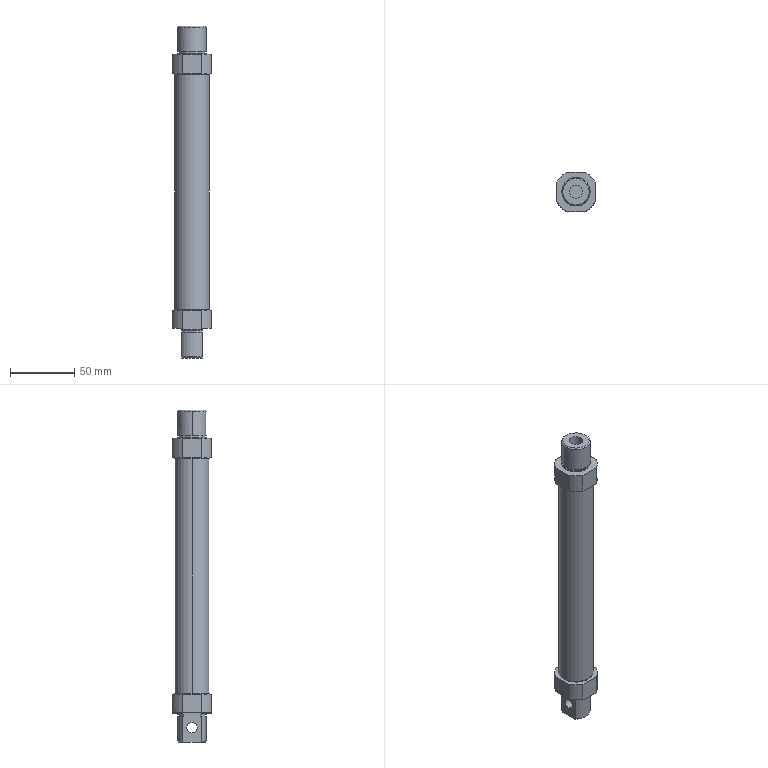Part | STEP file | fA_C85N25-100T(OUT)1 | 1 solid | 67 faces | box 30 x 30 x 257.5 mm | volume 131255 mm3 | cylinder 32 | plane 29 | cone 6 | commonest cylinder face diameters 22 x8 33.4 x8 20.37 x4 25.6 x4 8 x2 8.57 x2